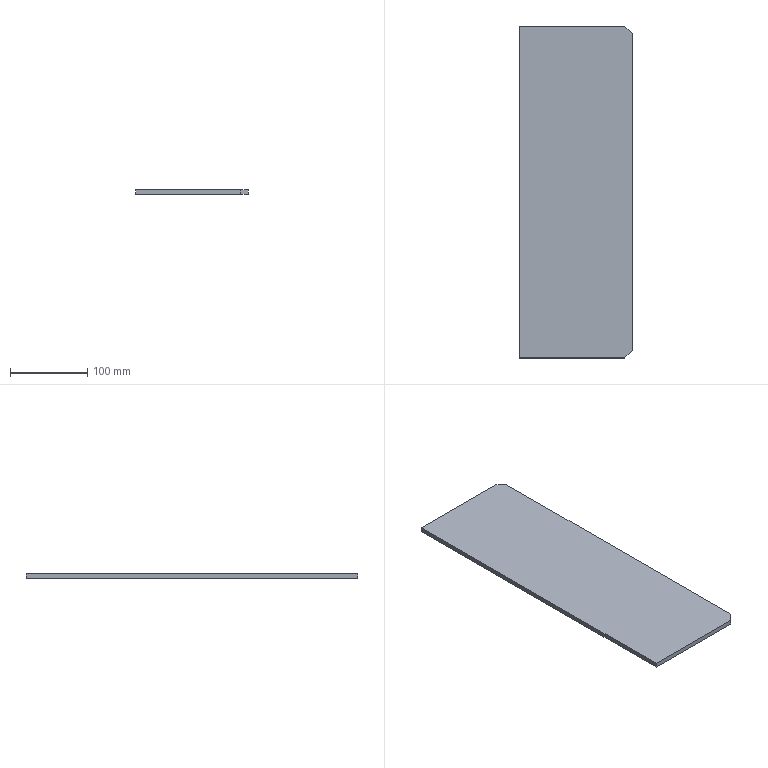Part | STEP file | 04-Rib plate 2 | 1 solid | 8 faces | box 146 x 429 x 6 mm | volume 375204 mm3 | plane 8
STEP:
#1=CARTESIAN_POINT('',(0.,0.,0.));
#2=DIRECTION('',(0.,0.,1.));
#3=DIRECTION('',(1.,0.,0.));
#4=AXIS2_PLACEMENT_3D('',#1,#2,#3);
#5=CARTESIAN_POINT('',(0.,0.,0.));
#6=VERTEX_POINT('',#5);
#7=CARTESIAN_POINT('',(0.,-429.,0.));
#8=VERTEX_POINT('',#7);
#9=CARTESIAN_POINT('',(0.,0.,0.));
#10=DIRECTION('',(0.,-1.,0.));
#11=VECTOR('',#10,1.);
#12=LINE('',#9,#11);
#13=CARTESIAN_POINT('',(0.,0.,6.));
#14=DIRECTION('',(1.,0.,0.));
#15=DIRECTION('',(0.,1.,0.));
#16=AXIS2_PLACEMENT_3D('',#13,#14,#15);
#17=PLANE('',#16);
#18=CARTESIAN_POINT('',(0.,-6.));
#19=DIRECTION('',(-1.,0.));
#20=VECTOR('',#19,1.);
#21=LINE('',#18,#20);
#22=(GEOMETRIC_REPRESENTATION_CONTEXT(2)PARAMETRIC_REPRESENTATION_CONTEXT()REPRESENTATION_CONTEXT('',''));
#23=DEFINITIONAL_REPRESENTATION('',(#21),#22);
#24=PCURVE('',#17,#23);
#25=CARTESIAN_POINT('',(0.,0.,0.));
#26=DIRECTION('',(0.,0.,1.));
#27=DIRECTION('',(1.,0.,0.));
#28=AXIS2_PLACEMENT_3D('',#25,#26,#27);
#29=PLANE('',#28);
#30=CARTESIAN_POINT('',(0.,0.));
#31=DIRECTION('',(0.,-1.));
#32=VECTOR('',#31,1.);
#33=LINE('',#30,#32);
#34=(GEOMETRIC_REPRESENTATION_CONTEXT(2)PARAMETRIC_REPRESENTATION_CONTEXT()REPRESENTATION_CONTEXT('',''));
#35=DEFINITIONAL_REPRESENTATION('',(#33),#34);
#36=PCURVE('',#29,#35);
#37=SURFACE_CURVE('',#12,(#24,#36),.PCURVE_S1.);
#38=EDGE_CURVE('',#6,#8,#37,.T.);
#39=ORIENTED_EDGE('',*,*,#38,.T.);
#40=CARTESIAN_POINT('',(0.,-429.,6.));
#41=VERTEX_POINT('',#40);
#42=CARTESIAN_POINT('',(0.,-429.,6.));
#43=DIRECTION('',(0.,0.,-1.));
#44=VECTOR('',#43,1.);
#45=LINE('',#42,#44);
#46=CARTESIAN_POINT('',(-429.,0.));
#47=DIRECTION('',(0.,-1.));
#48=VECTOR('',#47,1.);
#49=LINE('',#46,#48);
#50=(GEOMETRIC_REPRESENTATION_CONTEXT(2)PARAMETRIC_REPRESENTATION_CONTEXT()REPRESENTATION_CONTEXT('',''));
#51=DEFINITIONAL_REPRESENTATION('',(#49),#50);
#52=PCURVE('',#17,#51);
#53=CARTESIAN_POINT('',(0.,-429.,6.));
#54=DIRECTION('',(0.,1.,0.));
#55=DIRECTION('',(0.,0.,1.));
#56=AXIS2_PLACEMENT_3D('',#53,#54,#55);
#57=PLANE('',#56);
#58=CARTESIAN_POINT('',(0.,0.));
#59=DIRECTION('',(-1.,0.));
#60=VECTOR('',#59,1.);
#61=LINE('',#58,#60);
#62=(GEOMETRIC_REPRESENTATION_CONTEXT(2)PARAMETRIC_REPRESENTATION_CONTEXT()REPRESENTATION_CONTEXT('',''));
#63=DEFINITIONAL_REPRESENTATION('',(#61),#62);
#64=PCURVE('',#57,#63);
#65=SURFACE_CURVE('',#45,(#52,#64),.PCURVE_S1.);
#66=EDGE_CURVE('',#41,#8,#65,.T.);
#67=ORIENTED_EDGE('',*,*,#66,.F.);
#68=CARTESIAN_POINT('',(0.,0.,6.));
#69=VERTEX_POINT('',#68);
#70=CARTESIAN_POINT('',(0.,0.,6.));
#71=DIRECTION('',(0.,-1.,0.));
#72=VECTOR('',#71,1.);
#73=LINE('',#70,#72);
#74=CARTESIAN_POINT('',(0.,0.));
#75=DIRECTION('',(-1.,0.));
#76=VECTOR('',#75,1.);
#77=LINE('',#74,#76);
#78=(GEOMETRIC_REPRESENTATION_CONTEXT(2)PARAMETRIC_REPRESENTATION_CONTEXT()REPRESENTATION_CONTEXT('',''));
#79=DEFINITIONAL_REPRESENTATION('',(#77),#78);
#80=PCURVE('',#17,#79);
#81=CARTESIAN_POINT('',(0.,0.,6.));
#82=DIRECTION('',(0.,0.,1.));
#83=DIRECTION('',(1.,0.,0.));
#84=AXIS2_PLACEMENT_3D('',#81,#82,#83);
#85=PLANE('',#84);
#86=CARTESIAN_POINT('',(0.,0.));
#87=DIRECTION('',(0.,-1.));
#88=VECTOR('',#87,1.);
#89=LINE('',#86,#88);
#90=(GEOMETRIC_REPRESENTATION_CONTEXT(2)PARAMETRIC_REPRESENTATION_CONTEXT()REPRESENTATION_CONTEXT('',''));
#91=DEFINITIONAL_REPRESENTATION('',(#89),#90);
#92=PCURVE('',#85,#91);
#93=SURFACE_CURVE('',#73,(#80,#92),.PCURVE_S1.);
#94=EDGE_CURVE('',#69,#41,#93,.T.);
#95=ORIENTED_EDGE('',*,*,#94,.F.);
#96=CARTESIAN_POINT('',(0.,0.,6.));
#97=DIRECTION('',(0.,0.,-1.));
#98=VECTOR('',#97,1.);
#99=LINE('',#96,#98);
#100=CARTESIAN_POINT('',(0.,0.));
#101=DIRECTION('',(0.,-1.));
#102=VECTOR('',#101,1.);
#103=LINE('',#100,#102);
#104=(GEOMETRIC_REPRESENTATION_CONTEXT(2)PARAMETRIC_REPRESENTATION_CONTEXT()REPRESENTATION_CONTEXT('',''));
#105=DEFINITIONAL_REPRESENTATION('',(#103),#104);
#106=PCURVE('',#17,#105);
#107=CARTESIAN_POINT('',(0.,0.,6.));
#108=DIRECTION('',(0.,-1.,0.));
#109=DIRECTION('',(0.,0.,-1.));
#110=AXIS2_PLACEMENT_3D('',#107,#108,#109);
#111=PLANE('',#110);
#112=CARTESIAN_POINT('',(0.,0.));
#113=DIRECTION('',(1.,0.));
#114=VECTOR('',#113,1.);
#115=LINE('',#112,#114);
#116=(GEOMETRIC_REPRESENTATION_CONTEXT(2)PARAMETRIC_REPRESENTATION_CONTEXT()REPRESENTATION_CONTEXT('',''));
#117=DEFINITIONAL_REPRESENTATION('',(#115),#116);
#118=PCURVE('',#111,#117);
#119=SURFACE_CURVE('',#99,(#106,#118),.PCURVE_S1.);
#120=EDGE_CURVE('',#69,#6,#119,.T.);
#121=ORIENTED_EDGE('',*,*,#120,.T.);
#122=EDGE_LOOP('',(#39,#67,#95,#121));
#123=FACE_BOUND('',#122,.T.);
#124=ADVANCED_FACE('',(#123),#17,.F.);
#125=CARTESIAN_POINT('',(136.,-429.,0.));
#126=VERTEX_POINT('',#125);
#127=CARTESIAN_POINT('',(0.,-429.,0.));
#128=DIRECTION('',(1.,0.,0.));
#129=VECTOR('',#128,1.);
#130=LINE('',#127,#129);
#131=CARTESIAN_POINT('',(-6.,0.));
#132=DIRECTION('',(0.,1.));
#133=VECTOR('',#132,1.);
#134=LINE('',#131,#133);
#135=(GEOMETRIC_REPRESENTATION_CONTEXT(2)PARAMETRIC_REPRESENTATION_CONTEXT()REPRESENTATION_CONTEXT('',''));
#136=DEFINITIONAL_REPRESENTATION('',(#134),#135);
#137=PCURVE('',#57,#136);
#138=CARTESIAN_POINT('',(0.,-429.));
#139=DIRECTION('',(1.,0.));
#140=VECTOR('',#139,1.);
#141=LINE('',#138,#140);
#142=(GEOMETRIC_REPRESENTATION_CONTEXT(2)PARAMETRIC_REPRESENTATION_CONTEXT()REPRESENTATION_CONTEXT('',''));
#143=DEFINITIONAL_REPRESENTATION('',(#141),#142);
#144=PCURVE('',#29,#143);
#145=SURFACE_CURVE('',#130,(#137,#144),.PCURVE_S1.);
#146=EDGE_CURVE('',#8,#126,#145,.T.);
#147=ORIENTED_EDGE('',*,*,#146,.T.);
#148=CARTESIAN_POINT('',(136.,-429.,6.));
#149=VERTEX_POINT('',#148);
#150=CARTESIAN_POINT('',(136.,-429.,6.));
#151=DIRECTION('',(0.,0.,-1.));
#152=VECTOR('',#151,1.);
#153=LINE('',#150,#152);
#154=CARTESIAN_POINT('',(0.,136.));
#155=DIRECTION('',(-1.,0.));
#156=VECTOR('',#155,1.);
#157=LINE('',#154,#156);
#158=(GEOMETRIC_REPRESENTATION_CONTEXT(2)PARAMETRIC_REPRESENTATION_CONTEXT()REPRESENTATION_CONTEXT('',''));
#159=DEFINITIONAL_REPRESENTATION('',(#157),#158);
#160=PCURVE('',#57,#159);
#161=CARTESIAN_POINT('',(146.,-419.,6.));
#162=DIRECTION('',(-0.7071,0.7071,0.));
#163=DIRECTION('',(-0.7071,-0.7071,0.));
#164=AXIS2_PLACEMENT_3D('',#161,#162,#163);
#165=PLANE('',#164);
#166=CARTESIAN_POINT('',(14.142,0.));
#167=DIRECTION('',(0.,-1.));
#168=VECTOR('',#167,1.);
#169=LINE('',#166,#168);
#170=(GEOMETRIC_REPRESENTATION_CONTEXT(2)PARAMETRIC_REPRESENTATION_CONTEXT()REPRESENTATION_CONTEXT('',''));
#171=DEFINITIONAL_REPRESENTATION('',(#169),#170);
#172=PCURVE('',#165,#171);
#173=SURFACE_CURVE('',#153,(#160,#172),.PCURVE_S1.);
#174=EDGE_CURVE('',#149,#126,#173,.T.);
#175=ORIENTED_EDGE('',*,*,#174,.F.);
#176=CARTESIAN_POINT('',(0.,-429.,6.));
#177=DIRECTION('',(1.,0.,0.));
#178=VECTOR('',#177,1.);
#179=LINE('',#176,#178);
#180=CARTESIAN_POINT('',(0.,0.));
#181=DIRECTION('',(0.,1.));
#182=VECTOR('',#181,1.);
#183=LINE('',#180,#182);
#184=(GEOMETRIC_REPRESENTATION_CONTEXT(2)PARAMETRIC_REPRESENTATION_CONTEXT()REPRESENTATION_CONTEXT('',''));
#185=DEFINITIONAL_REPRESENTATION('',(#183),#184);
#186=PCURVE('',#57,#185);
#187=CARTESIAN_POINT('',(0.,-429.));
#188=DIRECTION('',(1.,0.));
#189=VECTOR('',#188,1.);
#190=LINE('',#187,#189);
#191=(GEOMETRIC_REPRESENTATION_CONTEXT(2)PARAMETRIC_REPRESENTATION_CONTEXT()REPRESENTATION_CONTEXT('',''));
#192=DEFINITIONAL_REPRESENTATION('',(#190),#191);
#193=PCURVE('',#85,#192);
#194=SURFACE_CURVE('',#179,(#186,#193),.PCURVE_S1.);
#195=EDGE_CURVE('',#41,#149,#194,.T.);
#196=ORIENTED_EDGE('',*,*,#195,.F.);
#197=ORIENTED_EDGE('',*,*,#66,.T.);
#198=EDGE_LOOP('',(#147,#175,#196,#197));
#199=FACE_BOUND('',#198,.T.);
#200=ADVANCED_FACE('',(#199),#57,.F.);
#201=CARTESIAN_POINT('',(146.,-419.,0.));
#202=VERTEX_POINT('',#201);
#203=CARTESIAN_POINT('',(146.,-419.,0.));
#204=DIRECTION('',(0.7071,0.7071,0.));
#205=VECTOR('',#204,1.);
#206=LINE('',#203,#205);
#207=CARTESIAN_POINT('',(0.,-6.));
#208=DIRECTION('',(-1.,0.));
#209=VECTOR('',#208,1.);
#210=LINE('',#207,#209);
#211=(GEOMETRIC_REPRESENTATION_CONTEXT(2)PARAMETRIC_REPRESENTATION_CONTEXT()REPRESENTATION_CONTEXT('',''));
#212=DEFINITIONAL_REPRESENTATION('',(#210),#211);
#213=PCURVE('',#165,#212);
#214=CARTESIAN_POINT('',(146.,-419.));
#215=DIRECTION('',(0.7071,0.7071));
#216=VECTOR('',#215,1.);
#217=LINE('',#214,#216);
#218=(GEOMETRIC_REPRESENTATION_CONTEXT(2)PARAMETRIC_REPRESENTATION_CONTEXT()REPRESENTATION_CONTEXT('',''));
#219=DEFINITIONAL_REPRESENTATION('',(#217),#218);
#220=PCURVE('',#29,#219);
#221=SURFACE_CURVE('',#206,(#213,#220),.PCURVE_S1.);
#222=EDGE_CURVE('',#126,#202,#221,.T.);
#223=ORIENTED_EDGE('',*,*,#222,.T.);
#224=CARTESIAN_POINT('',(146.,-419.,6.));
#225=VERTEX_POINT('',#224);
#226=CARTESIAN_POINT('',(146.,-419.,6.));
#227=DIRECTION('',(0.,0.,-1.));
#228=VECTOR('',#227,1.);
#229=LINE('',#226,#228);
#230=CARTESIAN_POINT('',(0.,0.));
#231=DIRECTION('',(0.,-1.));
#232=VECTOR('',#231,1.);
#233=LINE('',#230,#232);
#234=(GEOMETRIC_REPRESENTATION_CONTEXT(2)PARAMETRIC_REPRESENTATION_CONTEXT()REPRESENTATION_CONTEXT('',''));
#235=DEFINITIONAL_REPRESENTATION('',(#233),#234);
#236=PCURVE('',#165,#235);
#237=CARTESIAN_POINT('',(146.,-10.,6.));
#238=DIRECTION('',(-1.,0.,0.));
#239=DIRECTION('',(0.,-1.,0.));
#240=AXIS2_PLACEMENT_3D('',#237,#238,#239);
#241=PLANE('',#240);
#242=CARTESIAN_POINT('',(409.,0.));
#243=DIRECTION('',(0.,-1.));
#244=VECTOR('',#243,1.);
#245=LINE('',#242,#244);
#246=(GEOMETRIC_REPRESENTATION_CONTEXT(2)PARAMETRIC_REPRESENTATION_CONTEXT()REPRESENTATION_CONTEXT('',''));
#247=DEFINITIONAL_REPRESENTATION('',(#245),#246);
#248=PCURVE('',#241,#247);
#249=SURFACE_CURVE('',#229,(#236,#248),.PCURVE_S1.);
#250=EDGE_CURVE('',#225,#202,#249,.T.);
#251=ORIENTED_EDGE('',*,*,#250,.F.);
#252=CARTESIAN_POINT('',(146.,-419.,6.));
#253=DIRECTION('',(0.7071,0.7071,0.));
#254=VECTOR('',#253,1.);
#255=LINE('',#252,#254);
#256=CARTESIAN_POINT('',(0.,0.));
#257=DIRECTION('',(-1.,0.));
#258=VECTOR('',#257,1.);
#259=LINE('',#256,#258);
#260=(GEOMETRIC_REPRESENTATION_CONTEXT(2)PARAMETRIC_REPRESENTATION_CONTEXT()REPRESENTATION_CONTEXT('',''));
#261=DEFINITIONAL_REPRESENTATION('',(#259),#260);
#262=PCURVE('',#165,#261);
#263=CARTESIAN_POINT('',(146.,-419.));
#264=DIRECTION('',(0.7071,0.7071));
#265=VECTOR('',#264,1.);
#266=LINE('',#263,#265);
#267=(GEOMETRIC_REPRESENTATION_CONTEXT(2)PARAMETRIC_REPRESENTATION_CONTEXT()REPRESENTATION_CONTEXT('',''));
#268=DEFINITIONAL_REPRESENTATION('',(#266),#267);
#269=PCURVE('',#85,#268);
#270=SURFACE_CURVE('',#255,(#262,#269),.PCURVE_S1.);
#271=EDGE_CURVE('',#149,#225,#270,.T.);
#272=ORIENTED_EDGE('',*,*,#271,.F.);
#273=ORIENTED_EDGE('',*,*,#174,.T.);
#274=EDGE_LOOP('',(#223,#251,#272,#273));
#275=FACE_BOUND('',#274,.T.);
#276=ADVANCED_FACE('',(#275),#165,.F.);
#277=CARTESIAN_POINT('',(146.,-10.,0.));
#278=VERTEX_POINT('',#277);
#279=CARTESIAN_POINT('',(146.,-10.,0.));
#280=DIRECTION('',(0.,1.,0.));
#281=VECTOR('',#280,1.);
#282=LINE('',#279,#281);
#283=CARTESIAN_POINT('',(0.,-6.));
#284=DIRECTION('',(-1.,0.));
#285=VECTOR('',#284,1.);
#286=LINE('',#283,#285);
#287=(GEOMETRIC_REPRESENTATION_CONTEXT(2)PARAMETRIC_REPRESENTATION_CONTEXT()REPRESENTATION_CONTEXT('',''));
#288=DEFINITIONAL_REPRESENTATION('',(#286),#287);
#289=PCURVE('',#241,#288);
#290=CARTESIAN_POINT('',(146.,-10.));
#291=DIRECTION('',(0.,1.));
#292=VECTOR('',#291,1.);
#293=LINE('',#290,#292);
#294=(GEOMETRIC_REPRESENTATION_CONTEXT(2)PARAMETRIC_REPRESENTATION_CONTEXT()REPRESENTATION_CONTEXT('',''));
#295=DEFINITIONAL_REPRESENTATION('',(#293),#294);
#296=PCURVE('',#29,#295);
#297=SURFACE_CURVE('',#282,(#289,#296),.PCURVE_S1.);
#298=EDGE_CURVE('',#202,#278,#297,.T.);
#299=ORIENTED_EDGE('',*,*,#298,.T.);
#300=CARTESIAN_POINT('',(146.,-10.,6.));
#301=VERTEX_POINT('',#300);
#302=CARTESIAN_POINT('',(146.,-10.,6.));
#303=DIRECTION('',(0.,0.,-1.));
#304=VECTOR('',#303,1.);
#305=LINE('',#302,#304);
#306=CARTESIAN_POINT('',(0.,0.));
#307=DIRECTION('',(0.,-1.));
#308=VECTOR('',#307,1.);
#309=LINE('',#306,#308);
#310=(GEOMETRIC_REPRESENTATION_CONTEXT(2)PARAMETRIC_REPRESENTATION_CONTEXT()REPRESENTATION_CONTEXT('',''));
#311=DEFINITIONAL_REPRESENTATION('',(#309),#310);
#312=PCURVE('',#241,#311);
#313=CARTESIAN_POINT('',(136.,0.,6.));
#314=DIRECTION('',(-0.7071,-0.7071,0.));
#315=DIRECTION('',(0.7071,-0.7071,0.));
#316=AXIS2_PLACEMENT_3D('',#313,#314,#315);
#317=PLANE('',#316);
#318=CARTESIAN_POINT('',(14.142,0.));
#319=DIRECTION('',(0.,-1.));
#320=VECTOR('',#319,1.);
#321=LINE('',#318,#320);
#322=(GEOMETRIC_REPRESENTATION_CONTEXT(2)PARAMETRIC_REPRESENTATION_CONTEXT()REPRESENTATION_CONTEXT('',''));
#323=DEFINITIONAL_REPRESENTATION('',(#321),#322);
#324=PCURVE('',#317,#323);
#325=SURFACE_CURVE('',#305,(#312,#324),.PCURVE_S1.);
#326=EDGE_CURVE('',#301,#278,#325,.T.);
#327=ORIENTED_EDGE('',*,*,#326,.F.);
#328=CARTESIAN_POINT('',(146.,-10.,6.));
#329=DIRECTION('',(0.,1.,0.));
#330=VECTOR('',#329,1.);
#331=LINE('',#328,#330);
#332=CARTESIAN_POINT('',(0.,0.));
#333=DIRECTION('',(-1.,0.));
#334=VECTOR('',#333,1.);
#335=LINE('',#332,#334);
#336=(GEOMETRIC_REPRESENTATION_CONTEXT(2)PARAMETRIC_REPRESENTATION_CONTEXT()REPRESENTATION_CONTEXT('',''));
#337=DEFINITIONAL_REPRESENTATION('',(#335),#336);
#338=PCURVE('',#241,#337);
#339=CARTESIAN_POINT('',(146.,-10.));
#340=DIRECTION('',(0.,1.));
#341=VECTOR('',#340,1.);
#342=LINE('',#339,#341);
#343=(GEOMETRIC_REPRESENTATION_CONTEXT(2)PARAMETRIC_REPRESENTATION_CONTEXT()REPRESENTATION_CONTEXT('',''));
#344=DEFINITIONAL_REPRESENTATION('',(#342),#343);
#345=PCURVE('',#85,#344);
#346=SURFACE_CURVE('',#331,(#338,#345),.PCURVE_S1.);
#347=EDGE_CURVE('',#225,#301,#346,.T.);
#348=ORIENTED_EDGE('',*,*,#347,.F.);
#349=ORIENTED_EDGE('',*,*,#250,.T.);
#350=EDGE_LOOP('',(#299,#327,#348,#349));
#351=FACE_BOUND('',#350,.T.);
#352=ADVANCED_FACE('',(#351),#241,.F.);
#353=CARTESIAN_POINT('',(136.,0.,0.));
#354=VERTEX_POINT('',#353);
#355=CARTESIAN_POINT('',(136.,0.,0.));
#356=DIRECTION('',(-0.7071,0.7071,0.));
#357=VECTOR('',#356,1.);
#358=LINE('',#355,#357);
#359=CARTESIAN_POINT('',(0.,-6.));
#360=DIRECTION('',(-1.,0.));
#361=VECTOR('',#360,1.);
#362=LINE('',#359,#361);
#363=(GEOMETRIC_REPRESENTATION_CONTEXT(2)PARAMETRIC_REPRESENTATION_CONTEXT()REPRESENTATION_CONTEXT('',''));
#364=DEFINITIONAL_REPRESENTATION('',(#362),#363);
#365=PCURVE('',#317,#364);
#366=CARTESIAN_POINT('',(136.,0.));
#367=DIRECTION('',(-0.7071,0.7071));
#368=VECTOR('',#367,1.);
#369=LINE('',#366,#368);
#370=(GEOMETRIC_REPRESENTATION_CONTEXT(2)PARAMETRIC_REPRESENTATION_CONTEXT()REPRESENTATION_CONTEXT('',''));
#371=DEFINITIONAL_REPRESENTATION('',(#369),#370);
#372=PCURVE('',#29,#371);
#373=SURFACE_CURVE('',#358,(#365,#372),.PCURVE_S1.);
#374=EDGE_CURVE('',#278,#354,#373,.T.);
#375=ORIENTED_EDGE('',*,*,#374,.T.);
#376=CARTESIAN_POINT('',(136.,0.,6.));
#377=VERTEX_POINT('',#376);
#378=CARTESIAN_POINT('',(136.,0.,6.));
#379=DIRECTION('',(0.,0.,-1.));
#380=VECTOR('',#379,1.);
#381=LINE('',#378,#380);
#382=CARTESIAN_POINT('',(0.,0.));
#383=DIRECTION('',(0.,-1.));
#384=VECTOR('',#383,1.);
#385=LINE('',#382,#384);
#386=(GEOMETRIC_REPRESENTATION_CONTEXT(2)PARAMETRIC_REPRESENTATION_CONTEXT()REPRESENTATION_CONTEXT('',''));
#387=DEFINITIONAL_REPRESENTATION('',(#385),#386);
#388=PCURVE('',#317,#387);
#389=CARTESIAN_POINT('',(0.,136.));
#390=DIRECTION('',(1.,0.));
#391=VECTOR('',#390,1.);
#392=LINE('',#389,#391);
#393=(GEOMETRIC_REPRESENTATION_CONTEXT(2)PARAMETRIC_REPRESENTATION_CONTEXT()REPRESENTATION_CONTEXT('',''));
#394=DEFINITIONAL_REPRESENTATION('',(#392),#393);
#395=PCURVE('',#111,#394);
#396=SURFACE_CURVE('',#381,(#388,#395),.PCURVE_S1.);
#397=EDGE_CURVE('',#377,#354,#396,.T.);
#398=ORIENTED_EDGE('',*,*,#397,.F.);
#399=CARTESIAN_POINT('',(136.,0.,6.));
#400=DIRECTION('',(-0.7071,0.7071,0.));
#401=VECTOR('',#400,1.);
#402=LINE('',#399,#401);
#403=CARTESIAN_POINT('',(0.,0.));
#404=DIRECTION('',(-1.,0.));
#405=VECTOR('',#404,1.);
#406=LINE('',#403,#405);
#407=(GEOMETRIC_REPRESENTATION_CONTEXT(2)PARAMETRIC_REPRESENTATION_CONTEXT()REPRESENTATION_CONTEXT('',''));
#408=DEFINITIONAL_REPRESENTATION('',(#406),#407);
#409=PCURVE('',#317,#408);
#410=CARTESIAN_POINT('',(136.,0.));
#411=DIRECTION('',(-0.7071,0.7071));
#412=VECTOR('',#411,1.);
#413=LINE('',#410,#412);
#414=(GEOMETRIC_REPRESENTATION_CONTEXT(2)PARAMETRIC_REPRESENTATION_CONTEXT()REPRESENTATION_CONTEXT('',''));
#415=DEFINITIONAL_REPRESENTATION('',(#413),#414);
#416=PCURVE('',#85,#415);
#417=SURFACE_CURVE('',#402,(#409,#416),.PCURVE_S1.);
#418=EDGE_CURVE('',#301,#377,#417,.T.);
#419=ORIENTED_EDGE('',*,*,#418,.F.);
#420=ORIENTED_EDGE('',*,*,#326,.T.);
#421=EDGE_LOOP('',(#375,#398,#419,#420));
#422=FACE_BOUND('',#421,.T.);
#423=ADVANCED_FACE('',(#422),#317,.F.);
#424=CARTESIAN_POINT('',(0.,0.,0.));
#425=DIRECTION('',(-1.,0.,0.));
#426=VECTOR('',#425,1.);
#427=LINE('',#424,#426);
#428=CARTESIAN_POINT('',(6.,0.));
#429=DIRECTION('',(0.,-1.));
#430=VECTOR('',#429,1.);
#431=LINE('',#428,#430);
#432=(GEOMETRIC_REPRESENTATION_CONTEXT(2)PARAMETRIC_REPRESENTATION_CONTEXT()REPRESENTATION_CONTEXT('',''));
#433=DEFINITIONAL_REPRESENTATION('',(#431),#432);
#434=PCURVE('',#111,#433);
#435=CARTESIAN_POINT('',(0.,0.));
#436=DIRECTION('',(-1.,0.));
#437=VECTOR('',#436,1.);
#438=LINE('',#435,#437);
#439=(GEOMETRIC_REPRESENTATION_CONTEXT(2)PARAMETRIC_REPRESENTATION_CONTEXT()REPRESENTATION_CONTEXT('',''));
#440=DEFINITIONAL_REPRESENTATION('',(#438),#439);
#441=PCURVE('',#29,#440);
#442=SURFACE_CURVE('',#427,(#434,#441),.PCURVE_S1.);
#443=EDGE_CURVE('',#354,#6,#442,.T.);
#444=ORIENTED_EDGE('',*,*,#443,.T.);
#445=ORIENTED_EDGE('',*,*,#120,.F.);
#446=CARTESIAN_POINT('',(0.,0.,6.));
#447=DIRECTION('',(-1.,0.,0.));
#448=VECTOR('',#447,1.);
#449=LINE('',#446,#448);
#450=CARTESIAN_POINT('',(0.,0.));
#451=DIRECTION('',(0.,-1.));
#452=VECTOR('',#451,1.);
#453=LINE('',#450,#452);
#454=(GEOMETRIC_REPRESENTATION_CONTEXT(2)PARAMETRIC_REPRESENTATION_CONTEXT()REPRESENTATION_CONTEXT('',''));
#455=DEFINITIONAL_REPRESENTATION('',(#453),#454);
#456=PCURVE('',#111,#455);
#457=CARTESIAN_POINT('',(0.,0.));
#458=DIRECTION('',(-1.,0.));
#459=VECTOR('',#458,1.);
#460=LINE('',#457,#459);
#461=(GEOMETRIC_REPRESENTATION_CONTEXT(2)PARAMETRIC_REPRESENTATION_CONTEXT()REPRESENTATION_CONTEXT('',''));
#462=DEFINITIONAL_REPRESENTATION('',(#460),#461);
#463=PCURVE('',#85,#462);
#464=SURFACE_CURVE('',#449,(#456,#463),.PCURVE_S1.);
#465=EDGE_CURVE('',#377,#69,#464,.T.);
#466=ORIENTED_EDGE('',*,*,#465,.F.);
#467=ORIENTED_EDGE('',*,*,#397,.T.);
#468=EDGE_LOOP('',(#444,#445,#466,#467));
#469=FACE_BOUND('',#468,.T.);
#470=ADVANCED_FACE('',(#469),#111,.F.);
#471=ORIENTED_EDGE('',*,*,#94,.T.);
#472=ORIENTED_EDGE('',*,*,#195,.T.);
#473=ORIENTED_EDGE('',*,*,#271,.T.);
#474=ORIENTED_EDGE('',*,*,#347,.T.);
#475=ORIENTED_EDGE('',*,*,#418,.T.);
#476=ORIENTED_EDGE('',*,*,#465,.T.);
#477=EDGE_LOOP('',(#471,#472,#473,#474,#475,#476));
#478=FACE_BOUND('',#477,.T.);
#479=ADVANCED_FACE('',(#478),#85,.T.);
#480=ORIENTED_EDGE('',*,*,#38,.F.);
#481=ORIENTED_EDGE('',*,*,#443,.F.);
#482=ORIENTED_EDGE('',*,*,#374,.F.);
#483=ORIENTED_EDGE('',*,*,#298,.F.);
#484=ORIENTED_EDGE('',*,*,#222,.F.);
#485=ORIENTED_EDGE('',*,*,#146,.F.);
#486=EDGE_LOOP('',(#480,#481,#482,#483,#484,#485));
#487=FACE_BOUND('',#486,.T.);
#488=ADVANCED_FACE('',(#487),#29,.F.);
#489=CLOSED_SHELL('',(#124,#200,#276,#352,#423,#470,#479,#488));
#490=MANIFOLD_SOLID_BREP('',#489);
#491=(LENGTH_UNIT()NAMED_UNIT(*)SI_UNIT(.MILLI.,.METRE.));
#492=UNCERTAINTY_MEASURE_WITH_UNIT(LENGTH_MEASURE(0.0000001),#491,'','');
#493=(NAMED_UNIT(*)PLANE_ANGLE_UNIT()SI_UNIT($,.RADIAN.));
#494=(NAMED_UNIT(*)SI_UNIT($,.STERADIAN.)SOLID_ANGLE_UNIT());
#495=(GEOMETRIC_REPRESENTATION_CONTEXT(3)GLOBAL_UNCERTAINTY_ASSIGNED_CONTEXT((#492))GLOBAL_UNIT_ASSIGNED_CONTEXT((#491,#493,#494))REPRESENTATION_CONTEXT('',''));
#496=ADVANCED_BREP_SHAPE_REPRESENTATION('',(#4,#490),#495);